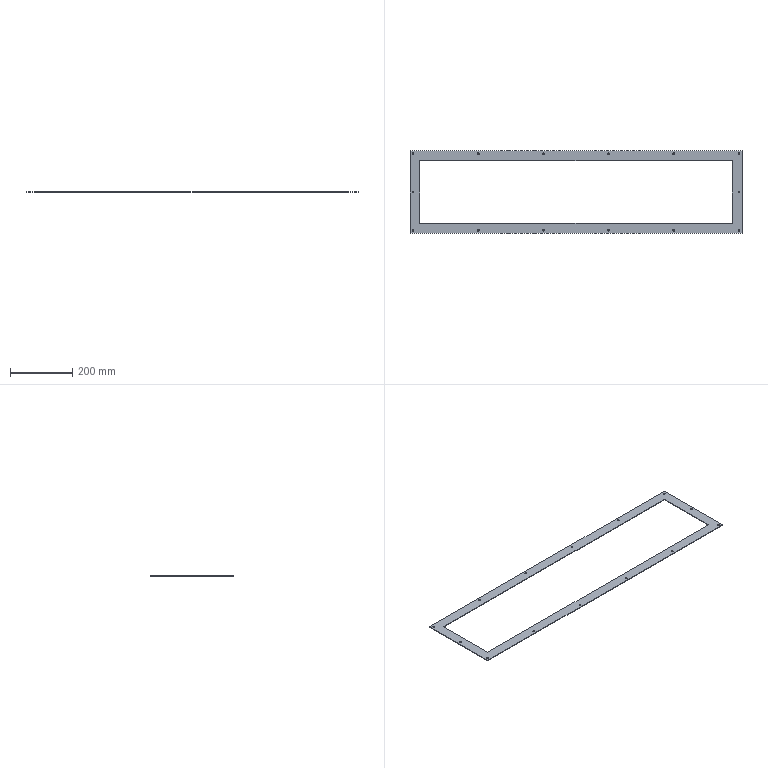Part | STEP file | 1 solid | 38 faces | box 1064 x 264 x 2 mm | volume 161000 mm3 | cylinder 28 | plane 10 | commonest cylinder face diameters 6 x28